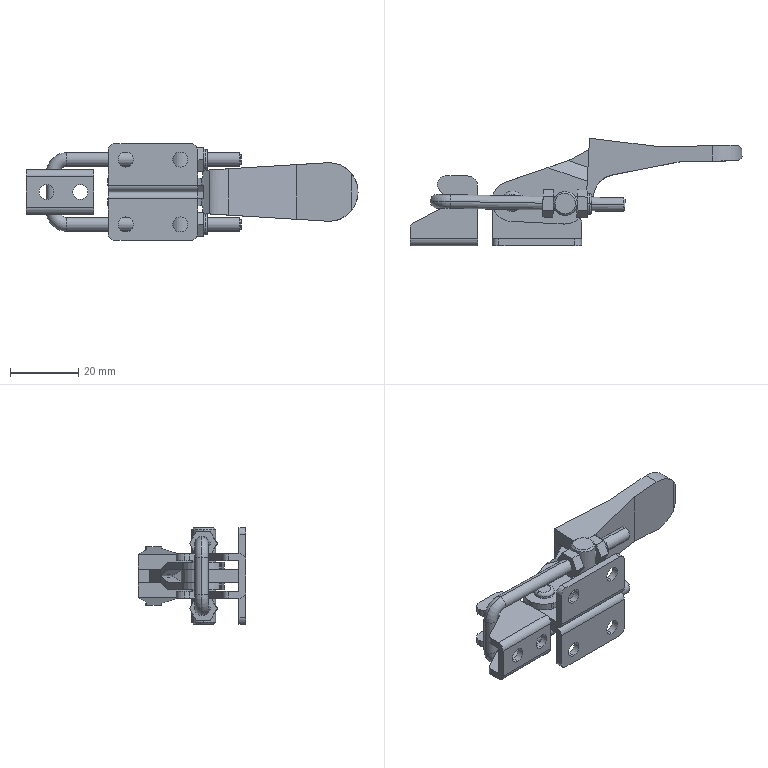Part | SolidWorks | 5 solids | 203 faces | box 97.135 x 31.44 x 28.2 mm | volume 12763 mm3 | plane 98 | cylinder 85 | torus 12 | cone 8 | commonest cylinder face diameters 4 x26 4.4 x12 5 x6 6 x6 7 x6 11.77 x6